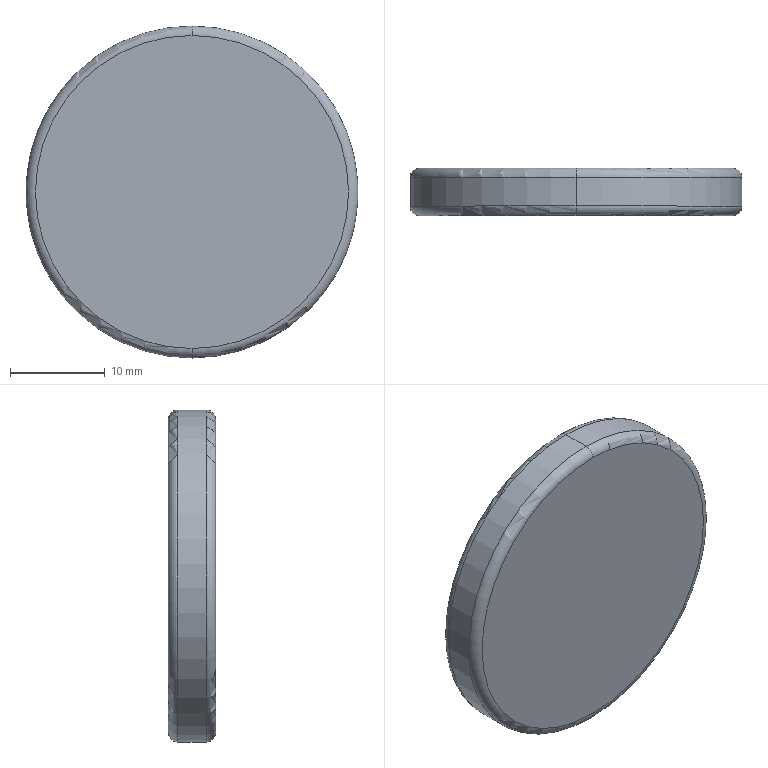Part | 1 solid | 8 faces | box 35 x 5 x 35 mm | volume 4764 mm3 | torus 4 | cylinder 2 | plane 2 | commonest cylinder face diameters 35 x2
STEP:
#1=CARTESIAN_POINT('',(0.,1.5,-17.5));
#2=VERTEX_POINT('',#1);
#3=CARTESIAN_POINT('',(0.,1.5,17.5));
#4=VERTEX_POINT('',#3);
#5=CARTESIAN_POINT('',(0.,1.5,0.));
#6=DIRECTION('',(0.,-1.,0.));
#7=DIRECTION('',(0.,0.,1.));
#8=AXIS2_PLACEMENT_3D('',#5,#6,#7);
#9=CIRCLE('',#8,17.5);
#10=EDGE_CURVE('',#2,#4,#9,.T.);
#11=ORIENTED_EDGE('',*,*,#10,.F.);
#12=CARTESIAN_POINT('',(0.,2.5,-16.5));
#13=VERTEX_POINT('',#12);
#14=CARTESIAN_POINT('',(0.,1.5,-16.5));
#15=DIRECTION('',(1.,0.,0.));
#16=DIRECTION('',(0.,0.,-1.));
#17=AXIS2_PLACEMENT_3D('',#14,#15,#16);
#18=CIRCLE('',#17,1.);
#19=EDGE_CURVE('',#2,#13,#18,.T.);
#20=ORIENTED_EDGE('',*,*,#19,.T.);
#21=CARTESIAN_POINT('',(0.,2.5,16.5));
#22=VERTEX_POINT('',#21);
#23=CARTESIAN_POINT('',(0.,2.5,0.));
#24=DIRECTION('',(0.,1.,0.));
#25=DIRECTION('',(0.,0.,1.));
#26=AXIS2_PLACEMENT_3D('',#23,#24,#25);
#27=CIRCLE('',#26,16.5);
#28=EDGE_CURVE('',#22,#13,#27,.T.);
#29=ORIENTED_EDGE('',*,*,#28,.F.);
#30=CARTESIAN_POINT('',(0.,1.5,16.5));
#31=DIRECTION('',(-1.,0.,0.));
#32=DIRECTION('',(0.,0.,1.));
#33=AXIS2_PLACEMENT_3D('',#30,#31,#32);
#34=CIRCLE('',#33,1.);
#35=EDGE_CURVE('',#4,#22,#34,.T.);
#36=ORIENTED_EDGE('',*,*,#35,.F.);
#37=EDGE_LOOP('',(#11,#20,#29,#36));
#38=FACE_OUTER_BOUND('',#37,.T.);
#39=CARTESIAN_POINT('',(0.,1.5,0.));
#40=DIRECTION('',(0.,1.,0.));
#41=DIRECTION('',(0.,0.,1.));
#42=AXIS2_PLACEMENT_3D('',#39,#40,#41);
#43=TOROIDAL_SURFACE('',#42,16.5,1.);
#44=ADVANCED_FACE('',(#38),#43,.T.);
#45=CARTESIAN_POINT('',(0.,-2.5,-16.5));
#46=VERTEX_POINT('',#45);
#47=CARTESIAN_POINT('',(0.,-2.5,16.5));
#48=VERTEX_POINT('',#47);
#49=CARTESIAN_POINT('',(0.,-2.5,0.));
#50=DIRECTION('',(0.,-1.,0.));
#51=DIRECTION('',(0.,0.,1.));
#52=AXIS2_PLACEMENT_3D('',#49,#50,#51);
#53=CIRCLE('',#52,16.5);
#54=EDGE_CURVE('',#46,#48,#53,.T.);
#55=ORIENTED_EDGE('',*,*,#54,.F.);
#56=CARTESIAN_POINT('',(0.,-1.5,-17.5));
#57=VERTEX_POINT('',#56);
#58=CARTESIAN_POINT('',(0.,-1.5,-16.5));
#59=DIRECTION('',(1.,0.,0.));
#60=DIRECTION('',(0.,0.,-1.));
#61=AXIS2_PLACEMENT_3D('',#58,#59,#60);
#62=CIRCLE('',#61,1.);
#63=EDGE_CURVE('',#46,#57,#62,.T.);
#64=ORIENTED_EDGE('',*,*,#63,.T.);
#65=CARTESIAN_POINT('',(0.,-1.5,17.5));
#66=VERTEX_POINT('',#65);
#67=CARTESIAN_POINT('',(0.,-1.5,0.));
#68=DIRECTION('',(0.,1.,0.));
#69=DIRECTION('',(0.,0.,1.));
#70=AXIS2_PLACEMENT_3D('',#67,#68,#69);
#71=CIRCLE('',#70,17.5);
#72=EDGE_CURVE('',#66,#57,#71,.T.);
#73=ORIENTED_EDGE('',*,*,#72,.F.);
#74=CARTESIAN_POINT('',(0.,-1.5,16.5));
#75=DIRECTION('',(-1.,0.,0.));
#76=DIRECTION('',(0.,0.,1.));
#77=AXIS2_PLACEMENT_3D('',#74,#75,#76);
#78=CIRCLE('',#77,1.);
#79=EDGE_CURVE('',#48,#66,#78,.T.);
#80=ORIENTED_EDGE('',*,*,#79,.F.);
#81=EDGE_LOOP('',(#55,#64,#73,#80));
#82=FACE_OUTER_BOUND('',#81,.T.);
#83=CARTESIAN_POINT('',(0.,-1.5,0.));
#84=DIRECTION('',(0.,1.,0.));
#85=DIRECTION('',(0.,0.,1.));
#86=AXIS2_PLACEMENT_3D('',#83,#84,#85);
#87=TOROIDAL_SURFACE('',#86,16.5,1.);
#88=ADVANCED_FACE('',(#82),#87,.T.);
#89=ORIENTED_EDGE('',*,*,#10,.T.);
#90=CARTESIAN_POINT('',(0.,2.5,17.5));
#91=DIRECTION('',(0.,-1.,0.));
#92=VECTOR('',#91,1000.);
#93=LINE('',#90,#92);
#94=EDGE_CURVE('',#4,#66,#93,.T.);
#95=ORIENTED_EDGE('',*,*,#94,.T.);
#96=ORIENTED_EDGE('',*,*,#72,.T.);
#97=CARTESIAN_POINT('',(0.,2.5,-17.5));
#98=DIRECTION('',(0.,-1.,0.));
#99=VECTOR('',#98,1000.);
#100=LINE('',#97,#99);
#101=EDGE_CURVE('',#2,#57,#100,.T.);
#102=ORIENTED_EDGE('',*,*,#101,.F.);
#103=EDGE_LOOP('',(#89,#95,#96,#102));
#104=FACE_OUTER_BOUND('',#103,.T.);
#105=CARTESIAN_POINT('',(0.,2.5,0.));
#106=DIRECTION('',(0.,-1.,0.));
#107=DIRECTION('',(0.,0.,-1.));
#108=AXIS2_PLACEMENT_3D('',#105,#106,#107);
#109=CYLINDRICAL_SURFACE('',#108,17.5);
#110=ADVANCED_FACE('',(#104),#109,.T.);
#111=ORIENTED_EDGE('',*,*,#94,.F.);
#112=CARTESIAN_POINT('',(0.,1.5,0.));
#113=DIRECTION('',(0.,-1.,0.));
#114=DIRECTION('',(0.,0.,1.));
#115=AXIS2_PLACEMENT_3D('',#112,#113,#114);
#116=CIRCLE('',#115,17.5);
#117=EDGE_CURVE('',#4,#2,#116,.T.);
#118=ORIENTED_EDGE('',*,*,#117,.T.);
#119=ORIENTED_EDGE('',*,*,#101,.T.);
#120=CARTESIAN_POINT('',(0.,-1.5,0.));
#121=DIRECTION('',(0.,1.,0.));
#122=DIRECTION('',(0.,0.,1.));
#123=AXIS2_PLACEMENT_3D('',#120,#121,#122);
#124=CIRCLE('',#123,17.5);
#125=EDGE_CURVE('',#57,#66,#124,.T.);
#126=ORIENTED_EDGE('',*,*,#125,.T.);
#127=EDGE_LOOP('',(#111,#118,#119,#126));
#128=FACE_OUTER_BOUND('',#127,.T.);
#129=CARTESIAN_POINT('',(0.,2.5,0.));
#130=DIRECTION('',(0.,-1.,0.));
#131=DIRECTION('',(0.,0.,-1.));
#132=AXIS2_PLACEMENT_3D('',#129,#130,#131);
#133=CYLINDRICAL_SURFACE('',#132,17.5);
#134=ADVANCED_FACE('',(#128),#133,.T.);
#135=ORIENTED_EDGE('',*,*,#28,.T.);
#136=CARTESIAN_POINT('',(0.,2.5,0.));
#137=DIRECTION('',(0.,1.,0.));
#138=DIRECTION('',(0.,0.,1.));
#139=AXIS2_PLACEMENT_3D('',#136,#137,#138);
#140=CIRCLE('',#139,16.5);
#141=EDGE_CURVE('',#13,#22,#140,.T.);
#142=ORIENTED_EDGE('',*,*,#141,.T.);
#143=EDGE_LOOP('',(#135,#142));
#144=FACE_OUTER_BOUND('',#143,.T.);
#145=CARTESIAN_POINT('',(0.,2.5,0.));
#146=DIRECTION('',(0.,1.,0.));
#147=DIRECTION('',(0.,0.,1.));
#148=AXIS2_PLACEMENT_3D('',#145,#146,#147);
#149=PLANE('',#148);
#150=ADVANCED_FACE('',(#144),#149,.T.);
#151=CARTESIAN_POINT('',(0.,-2.5,0.));
#152=DIRECTION('',(0.,-1.,0.));
#153=DIRECTION('',(0.,0.,1.));
#154=AXIS2_PLACEMENT_3D('',#151,#152,#153);
#155=CIRCLE('',#154,16.5);
#156=EDGE_CURVE('',#48,#46,#155,.T.);
#157=ORIENTED_EDGE('',*,*,#156,.T.);
#158=ORIENTED_EDGE('',*,*,#54,.T.);
#159=EDGE_LOOP('',(#157,#158));
#160=FACE_OUTER_BOUND('',#159,.T.);
#161=CARTESIAN_POINT('',(0.,-2.5,0.));
#162=DIRECTION('',(0.,1.,0.));
#163=DIRECTION('',(0.,0.,1.));
#164=AXIS2_PLACEMENT_3D('',#161,#162,#163);
#165=PLANE('',#164);
#166=ADVANCED_FACE('',(#160),#165,.F.);
#167=ORIENTED_EDGE('',*,*,#63,.F.);
#168=ORIENTED_EDGE('',*,*,#156,.F.);
#169=ORIENTED_EDGE('',*,*,#79,.T.);
#170=ORIENTED_EDGE('',*,*,#125,.F.);
#171=EDGE_LOOP('',(#167,#168,#169,#170));
#172=FACE_OUTER_BOUND('',#171,.T.);
#173=CARTESIAN_POINT('',(0.,-1.5,0.));
#174=DIRECTION('',(0.,1.,0.));
#175=DIRECTION('',(0.,0.,1.));
#176=AXIS2_PLACEMENT_3D('',#173,#174,#175);
#177=TOROIDAL_SURFACE('',#176,16.5,1.);
#178=ADVANCED_FACE('',(#172),#177,.T.);
#179=ORIENTED_EDGE('',*,*,#19,.F.);
#180=ORIENTED_EDGE('',*,*,#117,.F.);
#181=ORIENTED_EDGE('',*,*,#35,.T.);
#182=ORIENTED_EDGE('',*,*,#141,.F.);
#183=EDGE_LOOP('',(#179,#180,#181,#182));
#184=FACE_OUTER_BOUND('',#183,.T.);
#185=CARTESIAN_POINT('',(0.,1.5,0.));
#186=DIRECTION('',(0.,1.,0.));
#187=DIRECTION('',(0.,0.,1.));
#188=AXIS2_PLACEMENT_3D('',#185,#186,#187);
#189=TOROIDAL_SURFACE('',#188,16.5,1.);
#190=ADVANCED_FACE('',(#184),#189,.T.);
#191=CLOSED_SHELL('',(#44,#88,#110,#134,#150,#166,#178,#190));
#192=MANIFOLD_SOLID_BREP('',#191);
#193=CARTESIAN_POINT('',(0.,0.,0.));
#194=DIRECTION('',(0.,0.,1.));
#195=DIRECTION('',(1.,0.,0.));
#196=AXIS2_PLACEMENT_3D('',#193,#194,#195);
#197=(LENGTH_UNIT()NAMED_UNIT(*)SI_UNIT(.MILLI.,.METRE.));
#198=UNCERTAINTY_MEASURE_WITH_UNIT(LENGTH_MEASURE(0.00001),#197,'','');
#199=(NAMED_UNIT(*)PLANE_ANGLE_UNIT()SI_UNIT($,.RADIAN.));
#200=(NAMED_UNIT(*)SI_UNIT($,.STERADIAN.)SOLID_ANGLE_UNIT());
#201=(GEOMETRIC_REPRESENTATION_CONTEXT(3)GLOBAL_UNCERTAINTY_ASSIGNED_CONTEXT((#198))GLOBAL_UNIT_ASSIGNED_CONTEXT((#197,#199,#200))REPRESENTATION_CONTEXT('',''));
#202=ADVANCED_BREP_SHAPE_REPRESENTATION('',(#192,#196),#201);